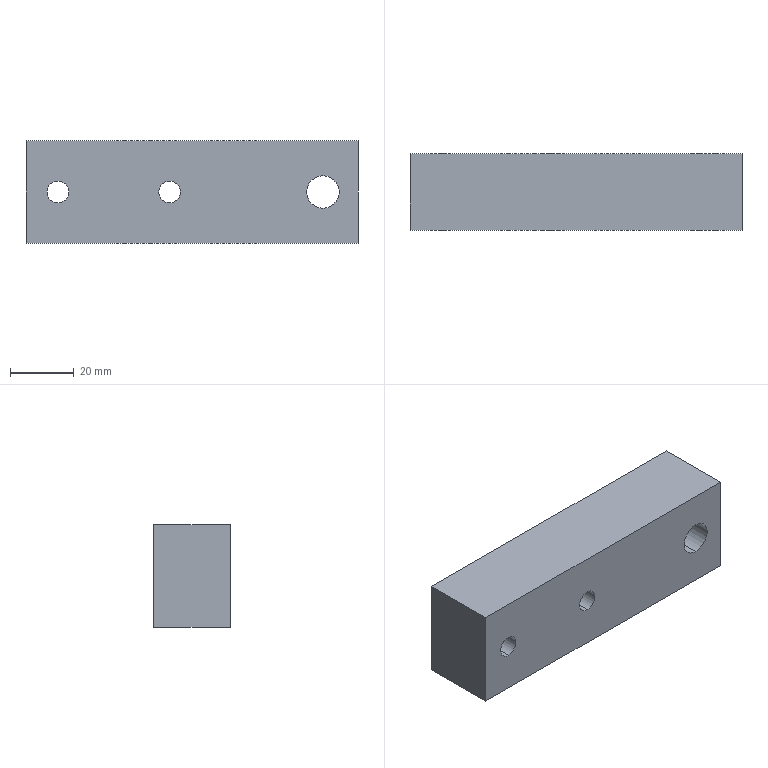Part | STEP file | PN_0030 (positioning fixed block) | 1 solid | 12 faces | box 104 x 24 x 32 mm | volume 76168 mm3 | cylinder 6 | plane 6 | commonest cylinder face diameters 6.8 x4 10.2 x2
STEP:
#1=CARTESIAN_POINT('',(0.,0.,0.));
#2=DIRECTION('',(0.,0.,1.));
#3=DIRECTION('',(1.,0.,0.));
#4=AXIS2_PLACEMENT_3D('',#1,#2,#3);
#5=CARTESIAN_POINT('',(10.,-12.,3.4));
#6=VERTEX_POINT('',#5);
#7=CARTESIAN_POINT('',(10.,12.,3.4));
#8=VERTEX_POINT('',#7);
#9=CARTESIAN_POINT('',(10.,12.,3.4));
#10=DIRECTION('',(0.,1.,0.));
#11=VECTOR('',#10,1.);
#12=LINE('',#9,#11);
#13=CARTESIAN_POINT('',(10.,12.,0.));
#14=DIRECTION('',(0.,1.,0.));
#15=DIRECTION('',(0.,0.,1.));
#16=AXIS2_PLACEMENT_3D('',#13,#14,#15);
#17=CYLINDRICAL_SURFACE('',#16,3.4);
#18=CARTESIAN_POINT('',(6.283,0.));
#19=DIRECTION('',(0.,1.));
#20=VECTOR('',#19,1.);
#21=LINE('',#18,#20);
#22=(GEOMETRIC_REPRESENTATION_CONTEXT(2)PARAMETRIC_REPRESENTATION_CONTEXT()REPRESENTATION_CONTEXT('',''));
#23=DEFINITIONAL_REPRESENTATION('',(#21),#22);
#24=PCURVE('',#17,#23);
#25=CARTESIAN_POINT('',(10.,12.,0.));
#26=DIRECTION('',(0.,1.,0.));
#27=DIRECTION('',(0.,0.,1.));
#28=AXIS2_PLACEMENT_3D('',#25,#26,#27);
#29=CYLINDRICAL_SURFACE('',#28,3.4);
#30=CARTESIAN_POINT('',(0.,0.));
#31=DIRECTION('',(0.,1.));
#32=VECTOR('',#31,1.);
#33=LINE('',#30,#32);
#34=(GEOMETRIC_REPRESENTATION_CONTEXT(2)PARAMETRIC_REPRESENTATION_CONTEXT()REPRESENTATION_CONTEXT('',''));
#35=DEFINITIONAL_REPRESENTATION('',(#33),#34);
#36=PCURVE('',#29,#35);
#37=SURFACE_CURVE('',#12,(#24,#36),.PCURVE_S1.);
#38=EDGE_CURVE('',#6,#8,#37,.T.);
#39=ORIENTED_EDGE('',*,*,#38,.T.);
#40=CARTESIAN_POINT('',(10.,12.,-3.4));
#41=VERTEX_POINT('',#40);
#42=CARTESIAN_POINT('',(10.,12.,0.));
#43=DIRECTION('',(0.,1.,0.));
#44=DIRECTION('',(0.,0.,1.));
#45=AXIS2_PLACEMENT_3D('',#42,#43,#44);
#46=CIRCLE('',#45,3.4);
#47=CARTESIAN_POINT('',(0.,0.));
#48=DIRECTION('',(1.,0.));
#49=VECTOR('',#48,1.);
#50=LINE('',#47,#49);
#51=(GEOMETRIC_REPRESENTATION_CONTEXT(2)PARAMETRIC_REPRESENTATION_CONTEXT()REPRESENTATION_CONTEXT('',''));
#52=DEFINITIONAL_REPRESENTATION('',(#50),#51);
#53=PCURVE('',#17,#52);
#54=CARTESIAN_POINT('',(0.,12.,16.));
#55=DIRECTION('',(0.,-1.,0.));
#56=DIRECTION('',(0.,0.,-1.));
#57=AXIS2_PLACEMENT_3D('',#54,#55,#56);
#58=PLANE('',#57);
#59=CARTESIAN_POINT('',(12.6,10.));
#60=CARTESIAN_POINT('',(12.6,15.889));
#61=CARTESIAN_POINT('',(17.7,12.944));
#62=CARTESIAN_POINT('',(22.8,10.));
#63=CARTESIAN_POINT('',(17.7,7.056));
#64=CARTESIAN_POINT('',(12.6,4.111));
#65=CARTESIAN_POINT('',(12.6,10.));
#66=(BOUNDED_CURVE()B_SPLINE_CURVE(2,(#59,#60,#61,#62,#63,#64,#65),.UNSPECIFIED.,.T.,.F.)B_SPLINE_CURVE_WITH_KNOTS((1,2,2,2,2,1),(-2.094,0.,2.094,4.189,6.283,8.378),.UNSPECIFIED.)CURVE()GEOMETRIC_REPRESENTATION_ITEM()RATIONAL_B_SPLINE_CURVE((1.,0.5,1.,0.5,1.,0.5,1.))REPRESENTATION_ITEM(''));
#67=(GEOMETRIC_REPRESENTATION_CONTEXT(2)PARAMETRIC_REPRESENTATION_CONTEXT()REPRESENTATION_CONTEXT('',''));
#68=DEFINITIONAL_REPRESENTATION('',(#66),#67);
#69=PCURVE('',#58,#68);
#70=SURFACE_CURVE('',#46,(#53,#69),.PCURVE_S1.);
#71=EDGE_CURVE('',#41,#8,#70,.T.);
#72=ORIENTED_EDGE('',*,*,#71,.F.);
#73=CARTESIAN_POINT('',(10.,-12.,-3.4));
#74=VERTEX_POINT('',#73);
#75=CARTESIAN_POINT('',(10.,12.,-3.4));
#76=DIRECTION('',(0.,1.,0.));
#77=VECTOR('',#76,1.);
#78=LINE('',#75,#77);
#79=CARTESIAN_POINT('',(3.142,0.));
#80=DIRECTION('',(0.,1.));
#81=VECTOR('',#80,1.);
#82=LINE('',#79,#81);
#83=(GEOMETRIC_REPRESENTATION_CONTEXT(2)PARAMETRIC_REPRESENTATION_CONTEXT()REPRESENTATION_CONTEXT('',''));
#84=DEFINITIONAL_REPRESENTATION('',(#82),#83);
#85=PCURVE('',#17,#84);
#86=CARTESIAN_POINT('',(3.142,0.));
#87=DIRECTION('',(0.,1.));
#88=VECTOR('',#87,1.);
#89=LINE('',#86,#88);
#90=(GEOMETRIC_REPRESENTATION_CONTEXT(2)PARAMETRIC_REPRESENTATION_CONTEXT()REPRESENTATION_CONTEXT('',''));
#91=DEFINITIONAL_REPRESENTATION('',(#89),#90);
#92=PCURVE('',#29,#91);
#93=SURFACE_CURVE('',#78,(#85,#92),.PCURVE_S1.);
#94=EDGE_CURVE('',#74,#41,#93,.T.);
#95=ORIENTED_EDGE('',*,*,#94,.F.);
#96=CARTESIAN_POINT('',(10.,-12.,0.));
#97=DIRECTION('',(0.,1.,0.));
#98=DIRECTION('',(0.,0.,1.));
#99=AXIS2_PLACEMENT_3D('',#96,#97,#98);
#100=CIRCLE('',#99,3.4);
#101=CARTESIAN_POINT('',(0.,-24.));
#102=DIRECTION('',(1.,0.));
#103=VECTOR('',#102,1.);
#104=LINE('',#101,#103);
#105=(GEOMETRIC_REPRESENTATION_CONTEXT(2)PARAMETRIC_REPRESENTATION_CONTEXT()REPRESENTATION_CONTEXT('',''));
#106=DEFINITIONAL_REPRESENTATION('',(#104),#105);
#107=PCURVE('',#17,#106);
#108=CARTESIAN_POINT('',(0.,-12.,16.));
#109=DIRECTION('',(0.,1.,0.));
#110=DIRECTION('',(0.,0.,1.));
#111=AXIS2_PLACEMENT_3D('',#108,#109,#110);
#112=PLANE('',#111);
#113=CARTESIAN_POINT('',(-16.,10.));
#114=DIRECTION('',(1.,0.));
#115=AXIS2_PLACEMENT_2D('',#113,#114);
#116=CIRCLE('',#115,3.4);
#117=(GEOMETRIC_REPRESENTATION_CONTEXT(2)PARAMETRIC_REPRESENTATION_CONTEXT()REPRESENTATION_CONTEXT('',''));
#118=DEFINITIONAL_REPRESENTATION('',(#116),#117);
#119=PCURVE('',#112,#118);
#120=SURFACE_CURVE('',#100,(#107,#119),.PCURVE_S1.);
#121=EDGE_CURVE('',#74,#6,#120,.T.);
#122=ORIENTED_EDGE('',*,*,#121,.T.);
#123=EDGE_LOOP('',(#39,#72,#95,#122));
#124=FACE_BOUND('',#123,.F.);
#125=ADVANCED_FACE('',(#124),#17,.F.);
#126=CARTESIAN_POINT('',(45.,-12.,3.4));
#127=VERTEX_POINT('',#126);
#128=CARTESIAN_POINT('',(45.,12.,3.4));
#129=VERTEX_POINT('',#128);
#130=CARTESIAN_POINT('',(45.,12.,3.4));
#131=DIRECTION('',(0.,1.,0.));
#132=VECTOR('',#131,1.);
#133=LINE('',#130,#132);
#134=CARTESIAN_POINT('',(45.,12.,0.));
#135=DIRECTION('',(0.,1.,0.));
#136=DIRECTION('',(0.,0.,1.));
#137=AXIS2_PLACEMENT_3D('',#134,#135,#136);
#138=CYLINDRICAL_SURFACE('',#137,3.4);
#139=CARTESIAN_POINT('',(6.283,0.));
#140=DIRECTION('',(0.,1.));
#141=VECTOR('',#140,1.);
#142=LINE('',#139,#141);
#143=(GEOMETRIC_REPRESENTATION_CONTEXT(2)PARAMETRIC_REPRESENTATION_CONTEXT()REPRESENTATION_CONTEXT('',''));
#144=DEFINITIONAL_REPRESENTATION('',(#142),#143);
#145=PCURVE('',#138,#144);
#146=CARTESIAN_POINT('',(45.,12.,0.));
#147=DIRECTION('',(0.,1.,0.));
#148=DIRECTION('',(0.,0.,1.));
#149=AXIS2_PLACEMENT_3D('',#146,#147,#148);
#150=CYLINDRICAL_SURFACE('',#149,3.4);
#151=CARTESIAN_POINT('',(0.,0.));
#152=DIRECTION('',(0.,1.));
#153=VECTOR('',#152,1.);
#154=LINE('',#151,#153);
#155=(GEOMETRIC_REPRESENTATION_CONTEXT(2)PARAMETRIC_REPRESENTATION_CONTEXT()REPRESENTATION_CONTEXT('',''));
#156=DEFINITIONAL_REPRESENTATION('',(#154),#155);
#157=PCURVE('',#150,#156);
#158=SURFACE_CURVE('',#133,(#145,#157),.PCURVE_S1.);
#159=EDGE_CURVE('',#127,#129,#158,.T.);
#160=ORIENTED_EDGE('',*,*,#159,.T.);
#161=CARTESIAN_POINT('',(45.,12.,-3.4));
#162=VERTEX_POINT('',#161);
#163=CARTESIAN_POINT('',(45.,12.,0.));
#164=DIRECTION('',(0.,1.,0.));
#165=DIRECTION('',(0.,0.,1.));
#166=AXIS2_PLACEMENT_3D('',#163,#164,#165);
#167=CIRCLE('',#166,3.4);
#168=CARTESIAN_POINT('',(0.,0.));
#169=DIRECTION('',(1.,0.));
#170=VECTOR('',#169,1.);
#171=LINE('',#168,#170);
#172=(GEOMETRIC_REPRESENTATION_CONTEXT(2)PARAMETRIC_REPRESENTATION_CONTEXT()REPRESENTATION_CONTEXT('',''));
#173=DEFINITIONAL_REPRESENTATION('',(#171),#172);
#174=PCURVE('',#138,#173);
#175=CARTESIAN_POINT('',(12.6,45.));
#176=CARTESIAN_POINT('',(12.6,50.889));
#177=CARTESIAN_POINT('',(17.7,47.944));
#178=CARTESIAN_POINT('',(22.8,45.));
#179=CARTESIAN_POINT('',(17.7,42.056));
#180=CARTESIAN_POINT('',(12.6,39.111));
#181=CARTESIAN_POINT('',(12.6,45.));
#182=(BOUNDED_CURVE()B_SPLINE_CURVE(2,(#175,#176,#177,#178,#179,#180,#181),.UNSPECIFIED.,.T.,.F.)B_SPLINE_CURVE_WITH_KNOTS((1,2,2,2,2,1),(-2.094,0.,2.094,4.189,6.283,8.378),.UNSPECIFIED.)CURVE()GEOMETRIC_REPRESENTATION_ITEM()RATIONAL_B_SPLINE_CURVE((1.,0.5,1.,0.5,1.,0.5,1.))REPRESENTATION_ITEM(''));
#183=(GEOMETRIC_REPRESENTATION_CONTEXT(2)PARAMETRIC_REPRESENTATION_CONTEXT()REPRESENTATION_CONTEXT('',''));
#184=DEFINITIONAL_REPRESENTATION('',(#182),#183);
#185=PCURVE('',#58,#184);
#186=SURFACE_CURVE('',#167,(#174,#185),.PCURVE_S1.);
#187=EDGE_CURVE('',#162,#129,#186,.T.);
#188=ORIENTED_EDGE('',*,*,#187,.F.);
#189=CARTESIAN_POINT('',(45.,-12.,-3.4));
#190=VERTEX_POINT('',#189);
#191=CARTESIAN_POINT('',(45.,12.,-3.4));
#192=DIRECTION('',(0.,1.,0.));
#193=VECTOR('',#192,1.);
#194=LINE('',#191,#193);
#195=CARTESIAN_POINT('',(3.142,0.));
#196=DIRECTION('',(0.,1.));
#197=VECTOR('',#196,1.);
#198=LINE('',#195,#197);
#199=(GEOMETRIC_REPRESENTATION_CONTEXT(2)PARAMETRIC_REPRESENTATION_CONTEXT()REPRESENTATION_CONTEXT('',''));
#200=DEFINITIONAL_REPRESENTATION('',(#198),#199);
#201=PCURVE('',#138,#200);
#202=CARTESIAN_POINT('',(3.142,0.));
#203=DIRECTION('',(0.,1.));
#204=VECTOR('',#203,1.);
#205=LINE('',#202,#204);
#206=(GEOMETRIC_REPRESENTATION_CONTEXT(2)PARAMETRIC_REPRESENTATION_CONTEXT()REPRESENTATION_CONTEXT('',''));
#207=DEFINITIONAL_REPRESENTATION('',(#205),#206);
#208=PCURVE('',#150,#207);
#209=SURFACE_CURVE('',#194,(#201,#208),.PCURVE_S1.);
#210=EDGE_CURVE('',#190,#162,#209,.T.);
#211=ORIENTED_EDGE('',*,*,#210,.F.);
#212=CARTESIAN_POINT('',(45.,-12.,0.));
#213=DIRECTION('',(0.,1.,0.));
#214=DIRECTION('',(0.,0.,1.));
#215=AXIS2_PLACEMENT_3D('',#212,#213,#214);
#216=CIRCLE('',#215,3.4);
#217=CARTESIAN_POINT('',(0.,-24.));
#218=DIRECTION('',(1.,0.));
#219=VECTOR('',#218,1.);
#220=LINE('',#217,#219);
#221=(GEOMETRIC_REPRESENTATION_CONTEXT(2)PARAMETRIC_REPRESENTATION_CONTEXT()REPRESENTATION_CONTEXT('',''));
#222=DEFINITIONAL_REPRESENTATION('',(#220),#221);
#223=PCURVE('',#138,#222);
#224=CARTESIAN_POINT('',(-16.,45.));
#225=DIRECTION('',(1.,0.));
#226=AXIS2_PLACEMENT_2D('',#224,#225);
#227=CIRCLE('',#226,3.4);
#228=(GEOMETRIC_REPRESENTATION_CONTEXT(2)PARAMETRIC_REPRESENTATION_CONTEXT()REPRESENTATION_CONTEXT('',''));
#229=DEFINITIONAL_REPRESENTATION('',(#227),#228);
#230=PCURVE('',#112,#229);
#231=SURFACE_CURVE('',#216,(#223,#230),.PCURVE_S1.);
#232=EDGE_CURVE('',#190,#127,#231,.T.);
#233=ORIENTED_EDGE('',*,*,#232,.T.);
#234=EDGE_LOOP('',(#160,#188,#211,#233));
#235=FACE_BOUND('',#234,.F.);
#236=ADVANCED_FACE('',(#235),#138,.F.);
#237=CARTESIAN_POINT('',(93.,-12.,5.1));
#238=VERTEX_POINT('',#237);
#239=CARTESIAN_POINT('',(93.,12.,5.1));
#240=VERTEX_POINT('',#239);
#241=CARTESIAN_POINT('',(93.,12.,5.1));
#242=DIRECTION('',(0.,1.,0.));
#243=VECTOR('',#242,1.);
#244=LINE('',#241,#243);
#245=CARTESIAN_POINT('',(93.,12.,0.));
#246=DIRECTION('',(0.,1.,0.));
#247=DIRECTION('',(0.,0.,1.));
#248=AXIS2_PLACEMENT_3D('',#245,#246,#247);
#249=CYLINDRICAL_SURFACE('',#248,5.1);
#250=CARTESIAN_POINT('',(6.283,0.));
#251=DIRECTION('',(0.,1.));
#252=VECTOR('',#251,1.);
#253=LINE('',#250,#252);
#254=(GEOMETRIC_REPRESENTATION_CONTEXT(2)PARAMETRIC_REPRESENTATION_CONTEXT()REPRESENTATION_CONTEXT('',''));
#255=DEFINITIONAL_REPRESENTATION('',(#253),#254);
#256=PCURVE('',#249,#255);
#257=CARTESIAN_POINT('',(93.,12.,0.));
#258=DIRECTION('',(0.,1.,0.));
#259=DIRECTION('',(0.,0.,1.));
#260=AXIS2_PLACEMENT_3D('',#257,#258,#259);
#261=CYLINDRICAL_SURFACE('',#260,5.1);
#262=CARTESIAN_POINT('',(0.,0.));
#263=DIRECTION('',(0.,1.));
#264=VECTOR('',#263,1.);
#265=LINE('',#262,#264);
#266=(GEOMETRIC_REPRESENTATION_CONTEXT(2)PARAMETRIC_REPRESENTATION_CONTEXT()REPRESENTATION_CONTEXT('',''));
#267=DEFINITIONAL_REPRESENTATION('',(#265),#266);
#268=PCURVE('',#261,#267);
#269=SURFACE_CURVE('',#244,(#256,#268),.PCURVE_S1.);
#270=EDGE_CURVE('',#238,#240,#269,.T.);
#271=ORIENTED_EDGE('',*,*,#270,.T.);
#272=CARTESIAN_POINT('',(93.,12.,-5.1));
#273=VERTEX_POINT('',#272);
#274=CARTESIAN_POINT('',(93.,12.,0.));
#275=DIRECTION('',(0.,1.,0.));
#276=DIRECTION('',(0.,0.,1.));
#277=AXIS2_PLACEMENT_3D('',#274,#275,#276);
#278=CIRCLE('',#277,5.1);
#279=CARTESIAN_POINT('',(0.,0.));
#280=DIRECTION('',(1.,0.));
#281=VECTOR('',#280,1.);
#282=LINE('',#279,#281);
#283=(GEOMETRIC_REPRESENTATION_CONTEXT(2)PARAMETRIC_REPRESENTATION_CONTEXT()REPRESENTATION_CONTEXT('',''));
#284=DEFINITIONAL_REPRESENTATION('',(#282),#283);
#285=PCURVE('',#249,#284);
#286=CARTESIAN_POINT('',(10.9,93.));
#287=CARTESIAN_POINT('',(10.9,101.833));
#288=CARTESIAN_POINT('',(18.55,97.417));
#289=CARTESIAN_POINT('',(26.2,93.));
#290=CARTESIAN_POINT('',(18.55,88.583));
#291=CARTESIAN_POINT('',(10.9,84.167));
#292=CARTESIAN_POINT('',(10.9,93.));
#293=(BOUNDED_CURVE()B_SPLINE_CURVE(2,(#286,#287,#288,#289,#290,#291,#292),.UNSPECIFIED.,.T.,.F.)B_SPLINE_CURVE_WITH_KNOTS((1,2,2,2,2,1),(-2.094,0.,2.094,4.189,6.283,8.378),.UNSPECIFIED.)CURVE()GEOMETRIC_REPRESENTATION_ITEM()RATIONAL_B_SPLINE_CURVE((1.,0.5,1.,0.5,1.,0.5,1.))REPRESENTATION_ITEM(''));
#294=(GEOMETRIC_REPRESENTATION_CONTEXT(2)PARAMETRIC_REPRESENTATION_CONTEXT()REPRESENTATION_CONTEXT('',''));
#295=DEFINITIONAL_REPRESENTATION('',(#293),#294);
#296=PCURVE('',#58,#295);
#297=SURFACE_CURVE('',#278,(#285,#296),.PCURVE_S1.);
#298=EDGE_CURVE('',#273,#240,#297,.T.);
#299=ORIENTED_EDGE('',*,*,#298,.F.);
#300=CARTESIAN_POINT('',(93.,-12.,-5.1));
#301=VERTEX_POINT('',#300);
#302=CARTESIAN_POINT('',(93.,12.,-5.1));
#303=DIRECTION('',(0.,1.,0.));
#304=VECTOR('',#303,1.);
#305=LINE('',#302,#304);
#306=CARTESIAN_POINT('',(3.142,0.));
#307=DIRECTION('',(0.,1.));
#308=VECTOR('',#307,1.);
#309=LINE('',#306,#308);
#310=(GEOMETRIC_REPRESENTATION_CONTEXT(2)PARAMETRIC_REPRESENTATION_CONTEXT()REPRESENTATION_CONTEXT('',''));
#311=DEFINITIONAL_REPRESENTATION('',(#309),#310);
#312=PCURVE('',#249,#311);
#313=CARTESIAN_POINT('',(3.142,0.));
#314=DIRECTION('',(0.,1.));
#315=VECTOR('',#314,1.);
#316=LINE('',#313,#315);
#317=(GEOMETRIC_REPRESENTATION_CONTEXT(2)PARAMETRIC_REPRESENTATION_CONTEXT()REPRESENTATION_CONTEXT('',''));
#318=DEFINITIONAL_REPRESENTATION('',(#316),#317);
#319=PCURVE('',#261,#318);
#320=SURFACE_CURVE('',#305,(#312,#319),.PCURVE_S1.);
#321=EDGE_CURVE('',#301,#273,#320,.T.);
#322=ORIENTED_EDGE('',*,*,#321,.F.);
#323=CARTESIAN_POINT('',(93.,-12.,0.));
#324=DIRECTION('',(0.,1.,0.));
#325=DIRECTION('',(0.,0.,1.));
#326=AXIS2_PLACEMENT_3D('',#323,#324,#325);
#327=CIRCLE('',#326,5.1);
#328=CARTESIAN_POINT('',(0.,-24.));
#329=DIRECTION('',(1.,0.));
#330=VECTOR('',#329,1.);
#331=LINE('',#328,#330);
#332=(GEOMETRIC_REPRESENTATION_CONTEXT(2)PARAMETRIC_REPRESENTATION_CONTEXT()REPRESENTATION_CONTEXT('',''));
#333=DEFINITIONAL_REPRESENTATION('',(#331),#332);
#334=PCURVE('',#249,#333);
#335=CARTESIAN_POINT('',(-16.,93.));
#336=DIRECTION('',(1.,0.));
#337=AXIS2_PLACEMENT_2D('',#335,#336);
#338=CIRCLE('',#337,5.1);
#339=(GEOMETRIC_REPRESENTATION_CONTEXT(2)PARAMETRIC_REPRESENTATION_CONTEXT()REPRESENTATION_CONTEXT('',''));
#340=DEFINITIONAL_REPRESENTATION('',(#338),#339);
#341=PCURVE('',#112,#340);
#342=SURFACE_CURVE('',#327,(#334,#341),.PCURVE_S1.);
#343=EDGE_CURVE('',#301,#238,#342,.T.);
#344=ORIENTED_EDGE('',*,*,#343,.T.);
#345=EDGE_LOOP('',(#271,#299,#322,#344));
#346=FACE_BOUND('',#345,.F.);
#347=ADVANCED_FACE('',(#346),#249,.F.);
#348=CARTESIAN_POINT('',(0.,12.,-16.));
#349=VERTEX_POINT('',#348);
#350=CARTESIAN_POINT('',(0.,-12.,-16.));
#351=VERTEX_POINT('',#350);
#352=CARTESIAN_POINT('',(0.,-12.,-16.));
#353=DIRECTION('',(0.,-1.,0.));
#354=VECTOR('',#353,1.);
#355=LINE('',#352,#354);
#356=CARTESIAN_POINT('',(0.,-12.,16.));
#357=DIRECTION('',(1.,0.,0.));
#358=DIRECTION('',(0.,0.,-1.));
#359=AXIS2_PLACEMENT_3D('',#356,#357,#358);
#360=PLANE('',#359);
#361=CARTESIAN_POINT('',(32.,0.));
#362=DIRECTION('',(0.,-1.));
#363=VECTOR('',#362,1.);
#364=LINE('',#361,#363);
#365=(GEOMETRIC_REPRESENTATION_CONTEXT(2)PARAMETRIC_REPRESENTATION_CONTEXT()REPRESENTATION_CONTEXT('',''));
#366=DEFINITIONAL_REPRESENTATION('',(#364),#365);
#367=PCURVE('',#360,#366);
#368=CARTESIAN_POINT('',(0.,0.,-16.));
#369=DIRECTION('',(0.,0.,-1.));
#370=DIRECTION('',(-1.,0.,0.));
#371=AXIS2_PLACEMENT_3D('',#368,#369,#370);
#372=PLANE('',#371);
#373=CARTESIAN_POINT('',(0.,-12.));
#374=DIRECTION('',(0.,-1.));
#375=VECTOR('',#374,1.);
#376=LINE('',#373,#375);
#377=(GEOMETRIC_REPRESENTATION_CONTEXT(2)PARAMETRIC_REPRESENTATION_CONTEXT()REPRESENTATION_CONTEXT('',''));
#378=DEFINITIONAL_REPRESENTATION('',(#376),#377);
#379=PCURVE('',#372,#378);
#380=SURFACE_CURVE('',#355,(#367,#379),.PCURVE_S1.);
#381=EDGE_CURVE('',#349,#351,#380,.T.);
#382=ORIENTED_EDGE('',*,*,#381,.T.);
#383=CARTESIAN_POINT('',(0.,-12.,16.));
#384=VERTEX_POINT('',#383);
#385=CARTESIAN_POINT('',(0.,-12.,16.));
#386=DIRECTION('',(0.,0.,-1.));
#387=VECTOR('',#386,1.);
#388=LINE('',#385,#387);
#389=CARTESIAN_POINT('',(0.,0.));
#390=DIRECTION('',(1.,0.));
#391=VECTOR('',#390,1.);
#392=LINE('',#389,#391);
#393=(GEOMETRIC_REPRESENTATION_CONTEXT(2)PARAMETRIC_REPRESENTATION_CONTEXT()REPRESENTATION_CONTEXT('',''));
#394=DEFINITIONAL_REPRESENTATION('',(#392),#393);
#395=PCURVE('',#360,#394);
#396=CARTESIAN_POINT('',(0.,0.));
#397=DIRECTION('',(-1.,0.));
#398=VECTOR('',#397,1.);
#399=LINE('',#396,#398);
#400=(GEOMETRIC_REPRESENTATION_CONTEXT(2)PARAMETRIC_REPRESENTATION_CONTEXT()REPRESENTATION_CONTEXT('',''));
#401=DEFINITIONAL_REPRESENTATION('',(#399),#400);
#402=PCURVE('',#112,#401);
#403=SURFACE_CURVE('',#388,(#395,#402),.PCURVE_S1.);
#404=EDGE_CURVE('',#384,#351,#403,.T.);
#405=ORIENTED_EDGE('',*,*,#404,.F.);
#406=CARTESIAN_POINT('',(0.,12.,16.));
#407=VERTEX_POINT('',#406);
#408=CARTESIAN_POINT('',(0.,-12.,16.));
#409=DIRECTION('',(0.,-1.,0.));
#410=VECTOR('',#409,1.);
#411=LINE('',#408,#410);
#412=CARTESIAN_POINT('',(0.,0.));
#413=DIRECTION('',(0.,-1.));
#414=VECTOR('',#413,1.);
#415=LINE('',#412,#414);
#416=(GEOMETRIC_REPRESENTATION_CONTEXT(2)PARAMETRIC_REPRESENTATION_CONTEXT()REPRESENTATION_CONTEXT('',''));
#417=DEFINITIONAL_REPRESENTATION('',(#415),#416);
#418=PCURVE('',#360,#417);
#419=CARTESIAN_POINT('',(0.,0.,16.));
#420=DIRECTION('',(0.,0.,-1.));
#421=DIRECTION('',(-1.,0.,0.));
#422=AXIS2_PLACEMENT_3D('',#419,#420,#421);
#423=PLANE('',#422);
#424=CARTESIAN_POINT('',(0.,-12.));
#425=DIRECTION('',(0.,-1.));
#426=VECTOR('',#425,1.);
#427=LINE('',#424,#426);
#428=(GEOMETRIC_REPRESENTATION_CONTEXT(2)PARAMETRIC_REPRESENTATION_CONTEXT()REPRESENTATION_CONTEXT('',''));
#429=DEFINITIONAL_REPRESENTATION('',(#427),#428);
#430=PCURVE('',#423,#429);
#431=SURFACE_CURVE('',#411,(#418,#430),.PCURVE_S1.);
#432=EDGE_CURVE('',#407,#384,#431,.T.);
#433=ORIENTED_EDGE('',*,*,#432,.F.);
#434=CARTESIAN_POINT('',(0.,12.,16.));
#435=DIRECTION('',(0.,0.,-1.));
#436=VECTOR('',#435,1.);
#437=LINE('',#434,#436);
#438=CARTESIAN_POINT('',(0.,24.));
#439=DIRECTION('',(1.,0.));
#440=VECTOR('',#439,1.);
#441=LINE('',#438,#440);
#442=(GEOMETRIC_REPRESENTATION_CONTEXT(2)PARAMETRIC_REPRESENTATION_CONTEXT()REPRESENTATION_CONTEXT('',''));
#443=DEFINITIONAL_REPRESENTATION('',(#441),#442);
#444=PCURVE('',#360,#443);
#445=CARTESIAN_POINT('',(0.,0.));
#446=DIRECTION('',(1.,0.));
#447=VECTOR('',#446,1.);
#448=LINE('',#445,#447);
#449=(GEOMETRIC_REPRESENTATION_CONTEXT(2)PARAMETRIC_REPRESENTATION_CONTEXT()REPRESENTATION_CONTEXT('',''));
#450=DEFINITIONAL_REPRESENTATION('',(#448),#449);
#451=PCURVE('',#58,#450);
#452=SURFACE_CURVE('',#437,(#444,#451),.PCURVE_S1.);
#453=EDGE_CURVE('',#407,#349,#452,.T.);
#454=ORIENTED_EDGE('',*,*,#453,.T.);
#455=EDGE_LOOP('',(#382,#405,#433,#454));
#456=FACE_BOUND('',#455,.T.);
#457=ADVANCED_FACE('',(#456),#360,.F.);
#458=CARTESIAN_POINT('',(10.,-12.,0.));
#459=DIRECTION('',(0.,1.,0.));
#460=DIRECTION('',(0.,0.,1.));
#461=AXIS2_PLACEMENT_3D('',#458,#459,#460);
#462=CIRCLE('',#461,3.4);
#463=CARTESIAN_POINT('',(-16.,10.));
#464=DIRECTION('',(1.,0.));
#465=AXIS2_PLACEMENT_2D('',#463,#464);
#466=CIRCLE('',#465,3.4);
#467=(GEOMETRIC_REPRESENTATION_CONTEXT(2)PARAMETRIC_REPRESENTATION_CONTEXT()REPRESENTATION_CONTEXT('',''));
#468=DEFINITIONAL_REPRESENTATION('',(#466),#467);
#469=PCURVE('',#112,#468);
#470=CARTESIAN_POINT('',(0.,-24.));
#471=DIRECTION('',(1.,0.));
#472=VECTOR('',#471,1.);
#473=LINE('',#470,#472);
#474=(GEOMETRIC_REPRESENTATION_CONTEXT(2)PARAMETRIC_REPRESENTATION_CONTEXT()REPRESENTATION_CONTEXT('',''));
#475=DEFINITIONAL_REPRESENTATION('',(#473),#474);
#476=PCURVE('',#29,#475);
#477=SURFACE_CURVE('',#462,(#469,#476),.PCURVE_S1.);
#478=EDGE_CURVE('',#6,#74,#477,.T.);
#479=ORIENTED_EDGE('',*,*,#478,.T.);
#480=ORIENTED_EDGE('',*,*,#121,.T.);
#481=EDGE_LOOP('',(#479,#480));
#482=FACE_BOUND('',#481,.T.);
#483=CARTESIAN_POINT('',(45.,-12.,0.));
#484=DIRECTION('',(0.,1.,0.));
#485=DIRECTION('',(0.,0.,1.));
#486=AXIS2_PLACEMENT_3D('',#483,#484,#485);
#487=CIRCLE('',#486,3.4);
#488=CARTESIAN_POINT('',(-16.,45.));
#489=DIRECTION('',(1.,0.));
#490=AXIS2_PLACEMENT_2D('',#488,#489);
#491=CIRCLE('',#490,3.4);
#492=(GEOMETRIC_REPRESENTATION_CONTEXT(2)PARAMETRIC_REPRESENTATION_CONTEXT()REPRESENTATION_CONTEXT('',''));
#493=DEFINITIONAL_REPRESENTATION('',(#491),#492);
#494=PCURVE('',#112,#493);
#495=CARTESIAN_POINT('',(0.,-24.));
#496=DIRECTION('',(1.,0.));
#497=VECTOR('',#496,1.);
#498=LINE('',#495,#497);
#499=(GEOMETRIC_REPRESENTATION_CONTEXT(2)PARAMETRIC_REPRESENTATION_CONTEXT()REPRESENTATION_CONTEXT('',''));
#500=DEFINITIONAL_REPRESENTATION('',(#498),#499);
#501=PCURVE('',#150,#500);
#502=SURFACE_CURVE('',#487,(#494,#501),.PCURVE_S1.);
#503=EDGE_CURVE('',#127,#190,#502,.T.);
#504=ORIENTED_EDGE('',*,*,#503,.T.);
#505=ORIENTED_EDGE('',*,*,#232,.T.);
#506=EDGE_LOOP('',(#504,#505));
#507=FACE_BOUND('',#506,.T.);
#508=CARTESIAN_POINT('',(93.,-12.,0.));
#509=DIRECTION('',(0.,1.,0.));
#510=DIRECTION('',(0.,0.,1.));
#511=AXIS2_PLACEMENT_3D('',#508,#509,#510);
#512=CIRCLE('',#511,5.1);
#513=CARTESIAN_POINT('',(-16.,93.));
#514=DIRECTION('',(1.,0.));
#515=AXIS2_PLACEMENT_2D('',#513,#514);
#516=CIRCLE('',#515,5.1);
#517=(GEOMETRIC_REPRESENTATION_CONTEXT(2)PARAMETRIC_REPRESENTATION_CONTEXT()REPRESENTATION_CONTEXT('',''));
#518=DEFINITIONAL_REPRESENTATION('',(#516),#517);
#519=PCURVE('',#112,#518);
#520=CARTESIAN_POINT('',(0.,-24.));
#521=DIRECTION('',(1.,0.));
#522=VECTOR('',#521,1.);
#523=LINE('',#520,#522);
#524=(GEOMETRIC_REPRESENTATION_CONTEXT(2)PARAMETRIC_REPRESENTATION_CONTEXT()REPRESENTATION_CONTEXT('',''));
#525=DEFINITIONAL_REPRESENTATION('',(#523),#524);
#526=PCURVE('',#261,#525);
#527=SURFACE_CURVE('',#512,(#519,#526),.PCURVE_S1.);
#528=EDGE_CURVE('',#238,#301,#527,.T.);
#529=ORIENTED_EDGE('',*,*,#528,.T.);
#530=ORIENTED_EDGE('',*,*,#343,.T.);
#531=EDGE_LOOP('',(#529,#530));
#532=FACE_BOUND('',#531,.T.);
#533=CARTESIAN_POINT('',(104.,-12.,-16.));
#534=VERTEX_POINT('',#533);
#535=CARTESIAN_POINT('',(0.,-12.,-16.));
#536=DIRECTION('',(1.,0.,0.));
#537=VECTOR('',#536,1.);
#538=LINE('',#535,#537);
#539=CARTESIAN_POINT('',(-32.,0.));
#540=DIRECTION('',(0.,1.));
#541=VECTOR('',#540,1.);
#542=LINE('',#539,#541);
#543=(GEOMETRIC_REPRESENTATION_CONTEXT(2)PARAMETRIC_REPRESENTATION_CONTEXT()REPRESENTATION_CONTEXT('',''));
#544=DEFINITIONAL_REPRESENTATION('',(#542),#543);
#545=PCURVE('',#112,#544);
#546=CARTESIAN_POINT('',(0.,-12.));
#547=DIRECTION('',(-1.,0.));
#548=VECTOR('',#547,1.);
#549=LINE('',#546,#548);
#550=(GEOMETRIC_REPRESENTATION_CONTEXT(2)PARAMETRIC_REPRESENTATION_CONTEXT()REPRESENTATION_CONTEXT('',''));
#551=DEFINITIONAL_REPRESENTATION('',(#549),#550);
#552=PCURVE('',#372,#551);
#553=SURFACE_CURVE('',#538,(#545,#552),.PCURVE_S1.);
#554=EDGE_CURVE('',#351,#534,#553,.T.);
#555=ORIENTED_EDGE('',*,*,#554,.T.);
#556=CARTESIAN_POINT('',(104.,-12.,16.));
#557=VERTEX_POINT('',#556);
#558=CARTESIAN_POINT('',(104.,-12.,16.));
#559=DIRECTION('',(0.,0.,-1.));
#560=VECTOR('',#559,1.);
#561=LINE('',#558,#560);
#562=CARTESIAN_POINT('',(0.,104.));
#563=DIRECTION('',(-1.,0.));
#564=VECTOR('',#563,1.);
#565=LINE('',#562,#564);
#566=(GEOMETRIC_REPRESENTATION_CONTEXT(2)PARAMETRIC_REPRESENTATION_CONTEXT()REPRESENTATION_CONTEXT('',''));
#567=DEFINITIONAL_REPRESENTATION('',(#565),#566);
#568=PCURVE('',#112,#567);
#569=CARTESIAN_POINT('',(104.,-12.,16.));
#570=DIRECTION('',(-1.,0.,0.));
#571=DIRECTION('',(0.,0.,1.));
#572=AXIS2_PLACEMENT_3D('',#569,#570,#571);
#573=PLANE('',#572);
#574=CARTESIAN_POINT('',(0.,0.));
#575=DIRECTION('',(-1.,0.));
#576=VECTOR('',#575,1.);
#577=LINE('',#574,#576);
#578=(GEOMETRIC_REPRESENTATION_CONTEXT(2)PARAMETRIC_REPRESENTATION_CONTEXT()REPRESENTATION_CONTEXT('',''));
#579=DEFINITIONAL_REPRESENTATION('',(#577),#578);
#580=PCURVE('',#573,#579);
#581=SURFACE_CURVE('',#561,(#568,#580),.PCURVE_S1.);
#582=EDGE_CURVE('',#557,#534,#581,.T.);
#583=ORIENTED_EDGE('',*,*,#582,.F.);
#584=CARTESIAN_POINT('',(0.,-12.,16.));
#585=DIRECTION('',(1.,0.,0.));
#586=VECTOR('',#585,1.);
#587=LINE('',#584,#586);
#588=CARTESIAN_POINT('',(0.,0.));
#589=DIRECTION('',(0.,1.));
#590=VECTOR('',#589,1.);
#591=LINE('',#588,#590);
#592=(GEOMETRIC_REPRESENTATION_CONTEXT(2)PARAMETRIC_REPRESENTATION_CONTEXT()REPRESENTATION_CONTEXT('',''));
#593=DEFINITIONAL_REPRESENTATION('',(#591),#592);
#594=PCURVE('',#112,#593);
#595=CARTESIAN_POINT('',(0.,-12.));
#596=DIRECTION('',(-1.,0.));
#597=VECTOR('',#596,1.);
#598=LINE('',#595,#597);
#599=(GEOMETRIC_REPRESENTATION_CONTEXT(2)PARAMETRIC_REPRESENTATION_CONTEXT()REPRESENTATION_CONTEXT('',''));
#600=DEFINITIONAL_REPRESENTATION('',(#598),#599);
#601=PCURVE('',#423,#600);
#602=SURFACE_CURVE('',#587,(#594,#601),.PCURVE_S1.);
#603=EDGE_CURVE('',#384,#557,#602,.T.);
#604=ORIENTED_EDGE('',*,*,#603,.F.);
#605=ORIENTED_EDGE('',*,*,#404,.T.);
#606=EDGE_LOOP('',(#555,#583,#604,#605));
#607=FACE_BOUND('',#606,.T.);
#608=ADVANCED_FACE('',(#482,#507,#532,#607),#112,.F.);
#609=CARTESIAN_POINT('',(104.,12.,-16.));
#610=VERTEX_POINT('',#609);
#611=CARTESIAN_POINT('',(104.,-12.,-16.));
#612=DIRECTION('',(0.,1.,0.));
#613=VECTOR('',#612,1.);
#614=LINE('',#611,#613);
#615=CARTESIAN_POINT('',(-32.,0.));
#616=DIRECTION('',(0.,1.));
#617=VECTOR('',#616,1.);
#618=LINE('',#615,#617);
#619=(GEOMETRIC_REPRESENTATION_CONTEXT(2)PARAMETRIC_REPRESENTATION_CONTEXT()REPRESENTATION_CONTEXT('',''));
#620=DEFINITIONAL_REPRESENTATION('',(#618),#619);
#621=PCURVE('',#573,#620);
#622=CARTESIAN_POINT('',(-104.,-12.));
#623=DIRECTION('',(0.,1.));
#624=VECTOR('',#623,1.);
#625=LINE('',#622,#624);
#626=(GEOMETRIC_REPRESENTATION_CONTEXT(2)PARAMETRIC_REPRESENTATION_CONTEXT()REPRESENTATION_CONTEXT('',''));
#627=DEFINITIONAL_REPRESENTATION('',(#625),#626);
#628=PCURVE('',#372,#627);
#629=SURFACE_CURVE('',#614,(#621,#628),.PCURVE_S1.);
#630=EDGE_CURVE('',#534,#610,#629,.T.);
#631=ORIENTED_EDGE('',*,*,#630,.T.);
#632=CARTESIAN_POINT('',(104.,12.,16.));
#633=VERTEX_POINT('',#632);
#634=CARTESIAN_POINT('',(104.,12.,16.));
#635=DIRECTION('',(0.,0.,-1.));
#636=VECTOR('',#635,1.);
#637=LINE('',#634,#636);
#638=CARTESIAN_POINT('',(0.,24.));
#639=DIRECTION('',(-1.,0.));
#640=VECTOR('',#639,1.);
#641=LINE('',#638,#640);
#642=(GEOMETRIC_REPRESENTATION_CONTEXT(2)PARAMETRIC_REPRESENTATION_CONTEXT()REPRESENTATION_CONTEXT('',''));
#643=DEFINITIONAL_REPRESENTATION('',(#641),#642);
#644=PCURVE('',#573,#643);
#645=CARTESIAN_POINT('',(0.,104.));
#646=DIRECTION('',(1.,0.));
#647=VECTOR('',#646,1.);
#648=LINE('',#645,#647);
#649=(GEOMETRIC_REPRESENTATION_CONTEXT(2)PARAMETRIC_REPRESENTATION_CONTEXT()REPRESENTATION_CONTEXT('',''));
#650=DEFINITIONAL_REPRESENTATION('',(#648),#649);
#651=PCURVE('',#58,#650);
#652=SURFACE_CURVE('',#637,(#644,#651),.PCURVE_S1.);
#653=EDGE_CURVE('',#633,#610,#652,.T.);
#654=ORIENTED_EDGE('',*,*,#653,.F.);
#655=CARTESIAN_POINT('',(104.,-12.,16.));
#656=DIRECTION('',(0.,1.,0.));
#657=VECTOR('',#656,1.);
#658=LINE('',#655,#657);
#659=CARTESIAN_POINT('',(0.,0.));
#660=DIRECTION('',(0.,1.));
#661=VECTOR('',#660,1.);
#662=LINE('',#659,#661);
#663=(GEOMETRIC_REPRESENTATION_CONTEXT(2)PARAMETRIC_REPRESENTATION_CONTEXT()REPRESENTATION_CONTEXT('',''));
#664=DEFINITIONAL_REPRESENTATION('',(#662),#663);
#665=PCURVE('',#573,#664);
#666=CARTESIAN_POINT('',(-104.,-12.));
#667=DIRECTION('',(0.,1.));
#668=VECTOR('',#667,1.);
#669=LINE('',#666,#668);
#670=(GEOMETRIC_REPRESENTATION_CONTEXT(2)PARAMETRIC_REPRESENTATION_CONTEXT()REPRESENTATION_CONTEXT('',''));
#671=DEFINITIONAL_REPRESENTATION('',(#669),#670);
#672=PCURVE('',#423,#671);
#673=SURFACE_CURVE('',#658,(#665,#672),.PCURVE_S1.);
#674=EDGE_CURVE('',#557,#633,#673,.T.);
#675=ORIENTED_EDGE('',*,*,#674,.F.);
#676=ORIENTED_EDGE('',*,*,#582,.T.);
#677=EDGE_LOOP('',(#631,#654,#675,#676));
#678=FACE_BOUND('',#677,.T.);
#679=ADVANCED_FACE('',(#678),#573,.F.);
#680=CARTESIAN_POINT('',(10.,12.,0.));
#681=DIRECTION('',(0.,1.,0.));
#682=DIRECTION('',(0.,0.,1.));
#683=AXIS2_PLACEMENT_3D('',#680,#681,#682);
#684=CIRCLE('',#683,3.4);
#685=CARTESIAN_POINT('',(12.6,10.));
#686=CARTESIAN_POINT('',(12.6,15.889));
#687=CARTESIAN_POINT('',(17.7,12.944));
#688=CARTESIAN_POINT('',(22.8,10.));
#689=CARTESIAN_POINT('',(17.7,7.056));
#690=CARTESIAN_POINT('',(12.6,4.111));
#691=CARTESIAN_POINT('',(12.6,10.));
#692=(BOUNDED_CURVE()B_SPLINE_CURVE(2,(#685,#686,#687,#688,#689,#690,#691),.UNSPECIFIED.,.T.,.F.)B_SPLINE_CURVE_WITH_KNOTS((1,2,2,2,2,1),(-2.094,0.,2.094,4.189,6.283,8.378),.UNSPECIFIED.)CURVE()GEOMETRIC_REPRESENTATION_ITEM()RATIONAL_B_SPLINE_CURVE((1.,0.5,1.,0.5,1.,0.5,1.))REPRESENTATION_ITEM(''));
#693=(GEOMETRIC_REPRESENTATION_CONTEXT(2)PARAMETRIC_REPRESENTATION_CONTEXT()REPRESENTATION_CONTEXT('',''));
#694=DEFINITIONAL_REPRESENTATION('',(#692),#693);
#695=PCURVE('',#58,#694);
#696=CARTESIAN_POINT('',(0.,0.));
#697=DIRECTION('',(1.,0.));
#698=VECTOR('',#697,1.);
#699=LINE('',#696,#698);
#700=(GEOMETRIC_REPRESENTATION_CONTEXT(2)PARAMETRIC_REPRESENTATION_CONTEXT()REPRESENTATION_CONTEXT('',''));
#701=DEFINITIONAL_REPRESENTATION('',(#699),#700);
#702=PCURVE('',#29,#701);
#703=SURFACE_CURVE('',#684,(#695,#702),.PCURVE_S1.);
#704=EDGE_CURVE('',#8,#41,#703,.T.);
#705=ORIENTED_EDGE('',*,*,#704,.F.);
#706=ORIENTED_EDGE('',*,*,#71,.F.);
#707=EDGE_LOOP('',(#705,#706));
#708=FACE_BOUND('',#707,.T.);
#709=CARTESIAN_POINT('',(45.,12.,0.));
#710=DIRECTION('',(0.,1.,0.));
#711=DIRECTION('',(0.,0.,1.));
#712=AXIS2_PLACEMENT_3D('',#709,#710,#711);
#713=CIRCLE('',#712,3.4);
#714=CARTESIAN_POINT('',(12.6,45.));
#715=CARTESIAN_POINT('',(12.6,50.889));
#716=CARTESIAN_POINT('',(17.7,47.944));
#717=CARTESIAN_POINT('',(22.8,45.));
#718=CARTESIAN_POINT('',(17.7,42.056));
#719=CARTESIAN_POINT('',(12.6,39.111));
#720=CARTESIAN_POINT('',(12.6,45.));
#721=(BOUNDED_CURVE()B_SPLINE_CURVE(2,(#714,#715,#716,#717,#718,#719,#720),.UNSPECIFIED.,.T.,.F.)B_SPLINE_CURVE_WITH_KNOTS((1,2,2,2,2,1),(-2.094,0.,2.094,4.189,6.283,8.378),.UNSPECIFIED.)CURVE()GEOMETRIC_REPRESENTATION_ITEM()RATIONAL_B_SPLINE_CURVE((1.,0.5,1.,0.5,1.,0.5,1.))REPRESENTATION_ITEM(''));
#722=(GEOMETRIC_REPRESENTATION_CONTEXT(2)PARAMETRIC_REPRESENTATION_CONTEXT()REPRESENTATION_CONTEXT('',''));
#723=DEFINITIONAL_REPRESENTATION('',(#721),#722);
#724=PCURVE('',#58,#723);
#725=CARTESIAN_POINT('',(0.,0.));
#726=DIRECTION('',(1.,0.));
#727=VECTOR('',#726,1.);
#728=LINE('',#725,#727);
#729=(GEOMETRIC_REPRESENTATION_CONTEXT(2)PARAMETRIC_REPRESENTATION_CONTEXT()REPRESENTATION_CONTEXT('',''));
#730=DEFINITIONAL_REPRESENTATION('',(#728),#729);
#731=PCURVE('',#150,#730);
#732=SURFACE_CURVE('',#713,(#724,#731),.PCURVE_S1.);
#733=EDGE_CURVE('',#129,#162,#732,.T.);
#734=ORIENTED_EDGE('',*,*,#733,.F.);
#735=ORIENTED_EDGE('',*,*,#187,.F.);
#736=EDGE_LOOP('',(#734,#735));
#737=FACE_BOUND('',#736,.T.);
#738=CARTESIAN_POINT('',(93.,12.,0.));
#739=DIRECTION('',(0.,1.,0.));
#740=DIRECTION('',(0.,0.,1.));
#741=AXIS2_PLACEMENT_3D('',#738,#739,#740);
#742=CIRCLE('',#741,5.1);
#743=CARTESIAN_POINT('',(10.9,93.));
#744=CARTESIAN_POINT('',(10.9,101.833));
#745=CARTESIAN_POINT('',(18.55,97.417));
#746=CARTESIAN_POINT('',(26.2,93.));
#747=CARTESIAN_POINT('',(18.55,88.583));
#748=CARTESIAN_POINT('',(10.9,84.167));
#749=CARTESIAN_POINT('',(10.9,93.));
#750=(BOUNDED_CURVE()B_SPLINE_CURVE(2,(#743,#744,#745,#746,#747,#748,#749),.UNSPECIFIED.,.T.,.F.)B_SPLINE_CURVE_WITH_KNOTS((1,2,2,2,2,1),(-2.094,0.,2.094,4.189,6.283,8.378),.UNSPECIFIED.)CURVE()GEOMETRIC_REPRESENTATION_ITEM()RATIONAL_B_SPLINE_CURVE((1.,0.5,1.,0.5,1.,0.5,1.))REPRESENTATION_ITEM(''));
#751=(GEOMETRIC_REPRESENTATION_CONTEXT(2)PARAMETRIC_REPRESENTATION_CONTEXT()REPRESENTATION_CONTEXT('',''));
#752=DEFINITIONAL_REPRESENTATION('',(#750),#751);
#753=PCURVE('',#58,#752);
#754=CARTESIAN_POINT('',(0.,0.));
#755=DIRECTION('',(1.,0.));
#756=VECTOR('',#755,1.);
#757=LINE('',#754,#756);
#758=(GEOMETRIC_REPRESENTATION_CONTEXT(2)PARAMETRIC_REPRESENTATION_CONTEXT()REPRESENTATION_CONTEXT('',''));
#759=DEFINITIONAL_REPRESENTATION('',(#757),#758);
#760=PCURVE('',#261,#759);
#761=SURFACE_CURVE('',#742,(#753,#760),.PCURVE_S1.);
#762=EDGE_CURVE('',#240,#273,#761,.T.);
#763=ORIENTED_EDGE('',*,*,#762,.F.);
#764=ORIENTED_EDGE('',*,*,#298,.F.);
#765=EDGE_LOOP('',(#763,#764));
#766=FACE_BOUND('',#765,.T.);
#767=CARTESIAN_POINT('',(0.,12.,-16.));
#768=DIRECTION('',(-1.,0.,0.));
#769=VECTOR('',#768,1.);
#770=LINE('',#767,#769);
#771=CARTESIAN_POINT('',(32.,0.));
#772=DIRECTION('',(0.,-1.));
#773=VECTOR('',#772,1.);
#774=LINE('',#771,#773);
#775=(GEOMETRIC_REPRESENTATION_CONTEXT(2)PARAMETRIC_REPRESENTATION_CONTEXT()REPRESENTATION_CONTEXT('',''));
#776=DEFINITIONAL_REPRESENTATION('',(#774),#775);
#777=PCURVE('',#58,#776);
#778=CARTESIAN_POINT('',(0.,12.));
#779=DIRECTION('',(1.,0.));
#780=VECTOR('',#779,1.);
#781=LINE('',#778,#780);
#782=(GEOMETRIC_REPRESENTATION_CONTEXT(2)PARAMETRIC_REPRESENTATION_CONTEXT()REPRESENTATION_CONTEXT('',''));
#783=DEFINITIONAL_REPRESENTATION('',(#781),#782);
#784=PCURVE('',#372,#783);
#785=SURFACE_CURVE('',#770,(#777,#784),.PCURVE_S1.);
#786=EDGE_CURVE('',#610,#349,#785,.T.);
#787=ORIENTED_EDGE('',*,*,#786,.T.);
#788=ORIENTED_EDGE('',*,*,#453,.F.);
#789=CARTESIAN_POINT('',(0.,12.,16.));
#790=DIRECTION('',(-1.,0.,0.));
#791=VECTOR('',#790,1.);
#792=LINE('',#789,#791);
#793=CARTESIAN_POINT('',(0.,0.));
#794=DIRECTION('',(0.,-1.));
#795=VECTOR('',#794,1.);
#796=LINE('',#793,#795);
#797=(GEOMETRIC_REPRESENTATION_CONTEXT(2)PARAMETRIC_REPRESENTATION_CONTEXT()REPRESENTATION_CONTEXT('',''));
#798=DEFINITIONAL_REPRESENTATION('',(#796),#797);
#799=PCURVE('',#58,#798);
#800=CARTESIAN_POINT('',(0.,12.));
#801=DIRECTION('',(1.,0.));
#802=VECTOR('',#801,1.);
#803=LINE('',#800,#802);
#804=(GEOMETRIC_REPRESENTATION_CONTEXT(2)PARAMETRIC_REPRESENTATION_CONTEXT()REPRESENTATION_CONTEXT('',''));
#805=DEFINITIONAL_REPRESENTATION('',(#803),#804);
#806=PCURVE('',#423,#805);
#807=SURFACE_CURVE('',#792,(#799,#806),.PCURVE_S1.);
#808=EDGE_CURVE('',#633,#407,#807,.T.);
#809=ORIENTED_EDGE('',*,*,#808,.F.);
#810=ORIENTED_EDGE('',*,*,#653,.T.);
#811=EDGE_LOOP('',(#787,#788,#809,#810));
#812=FACE_BOUND('',#811,.T.);
#813=ADVANCED_FACE('',(#708,#737,#766,#812),#58,.F.);
#814=ORIENTED_EDGE('',*,*,#432,.T.);
#815=ORIENTED_EDGE('',*,*,#603,.T.);
#816=ORIENTED_EDGE('',*,*,#674,.T.);
#817=ORIENTED_EDGE('',*,*,#808,.T.);
#818=EDGE_LOOP('',(#814,#815,#816,#817));
#819=FACE_BOUND('',#818,.T.);
#820=ADVANCED_FACE('',(#819),#423,.F.);
#821=ORIENTED_EDGE('',*,*,#381,.F.);
#822=ORIENTED_EDGE('',*,*,#786,.F.);
#823=ORIENTED_EDGE('',*,*,#630,.F.);
#824=ORIENTED_EDGE('',*,*,#554,.F.);
#825=EDGE_LOOP('',(#821,#822,#823,#824));
#826=FACE_BOUND('',#825,.T.);
#827=ADVANCED_FACE('',(#826),#372,.T.);
#828=ORIENTED_EDGE('',*,*,#762,.F.);
#829=ORIENTED_EDGE('',*,*,#270,.F.);
#830=ORIENTED_EDGE('',*,*,#528,.T.);
#831=ORIENTED_EDGE('',*,*,#321,.T.);
#832=EDGE_LOOP('',(#828,#829,#830,#831));
#833=FACE_BOUND('',#832,.F.);
#834=ADVANCED_FACE('',(#833),#261,.F.);
#835=ORIENTED_EDGE('',*,*,#733,.F.);
#836=ORIENTED_EDGE('',*,*,#159,.F.);
#837=ORIENTED_EDGE('',*,*,#503,.T.);
#838=ORIENTED_EDGE('',*,*,#210,.T.);
#839=EDGE_LOOP('',(#835,#836,#837,#838));
#840=FACE_BOUND('',#839,.F.);
#841=ADVANCED_FACE('',(#840),#150,.F.);
#842=ORIENTED_EDGE('',*,*,#704,.F.);
#843=ORIENTED_EDGE('',*,*,#38,.F.);
#844=ORIENTED_EDGE('',*,*,#478,.T.);
#845=ORIENTED_EDGE('',*,*,#94,.T.);
#846=EDGE_LOOP('',(#842,#843,#844,#845));
#847=FACE_BOUND('',#846,.F.);
#848=ADVANCED_FACE('',(#847),#29,.F.);
#849=CLOSED_SHELL('',(#125,#236,#347,#457,#608,#679,#813,#820,#827,#834,#841,#848));
#850=MANIFOLD_SOLID_BREP('',#849);
#851=(LENGTH_UNIT()NAMED_UNIT(*)SI_UNIT(.MILLI.,.METRE.));
#852=UNCERTAINTY_MEASURE_WITH_UNIT(LENGTH_MEASURE(0.0000001),#851,'','');
#853=(NAMED_UNIT(*)PLANE_ANGLE_UNIT()SI_UNIT($,.RADIAN.));
#854=(NAMED_UNIT(*)SI_UNIT($,.STERADIAN.)SOLID_ANGLE_UNIT());
#855=(GEOMETRIC_REPRESENTATION_CONTEXT(3)GLOBAL_UNCERTAINTY_ASSIGNED_CONTEXT((#852))GLOBAL_UNIT_ASSIGNED_CONTEXT((#851,#853,#854))REPRESENTATION_CONTEXT('',''));
#856=ADVANCED_BREP_SHAPE_REPRESENTATION('',(#4,#850),#855);